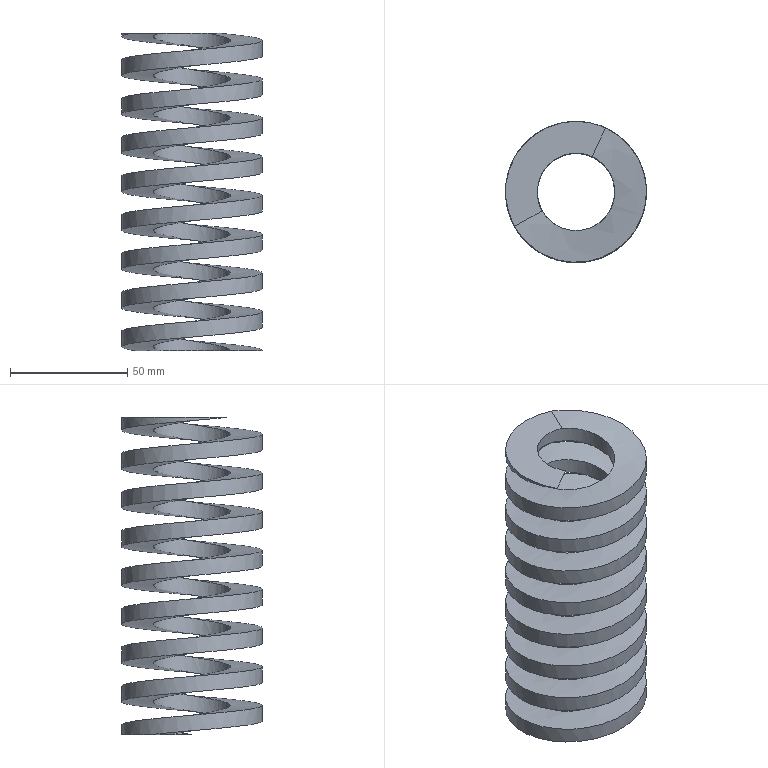Part | NX | features 模具.stp<1>[78] 2 | 1 solid | 5 faces | box 60.001 x 60 x 135.006 mm | volume 50788 mm3 | spline 2 | plane 2 | cylinder 1 | commonest cylinder face diameters 60 x1